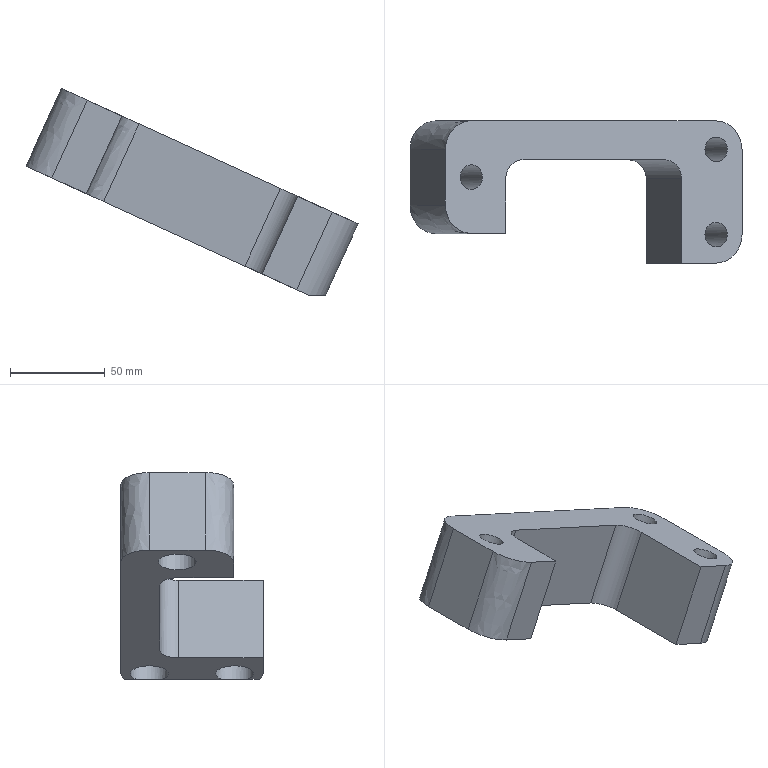Part | STEP file | solid 195 | 1 solid | 26 faces | box 175.156 x 75 x 109.18 mm | volume 273394 mm3 | plane 11 | cylinder 9 | spline 6 | commonest cylinder face diameters 20 x4 13 x3 30 x2